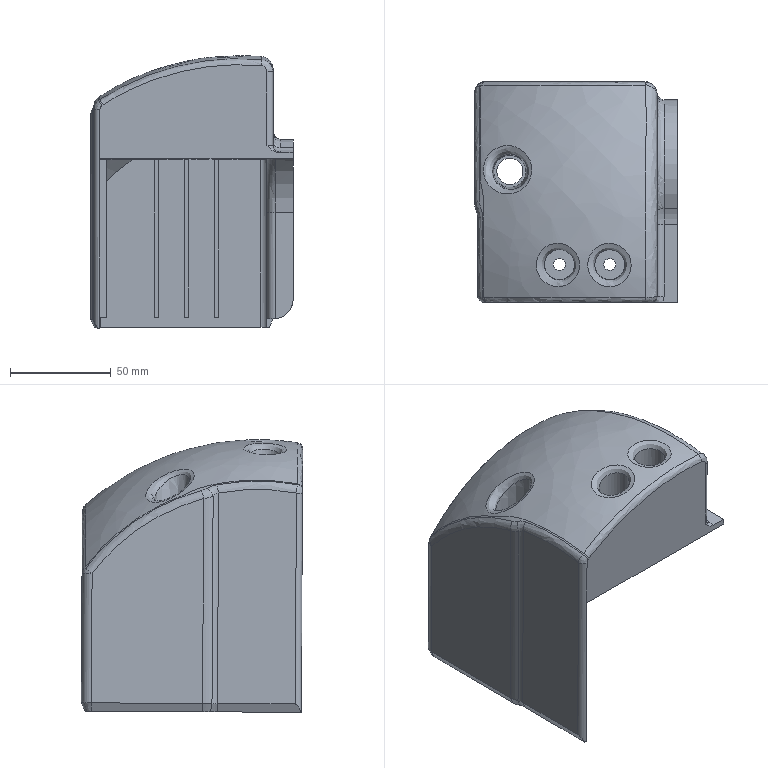Part | STEP file | EDN CAP NQ7AL | 1 solid | 148 faces | box 100.427 x 109.896 x 135.338 mm | volume 140123 mm3 | plane 79 | spline 32 | cylinder 31 | cone 4 | torus 2 | commonest cylinder face diameters 20 x8 6 x5 8 x3 13 x3 15 x2 4 x1